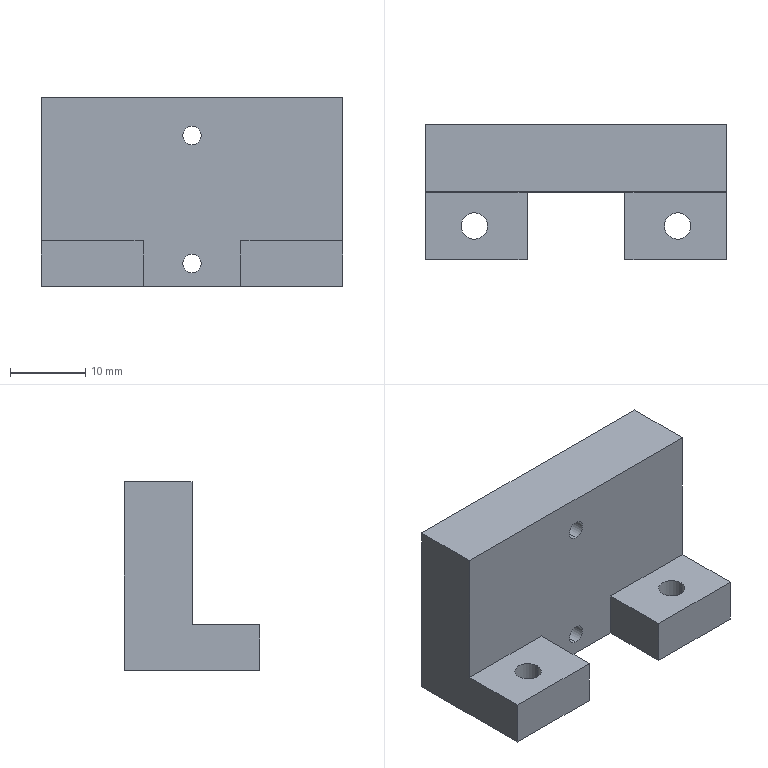Part | SolidWorks | features BaseBody 1 | 1 solid | 20 faces | box 40 x 18 x 25 mm | volume 10257 mm3 | plane 12 | cylinder 8 | commonest cylinder face diameters 2.459 x4 3.5 x4
STEP:
#1=CARTESIAN_POINT('',(-20.,18.,21.23));
#2=VERTEX_POINT('',#1);
#3=CARTESIAN_POINT('',(-20.,18.,18.77));
#4=VERTEX_POINT('',#3);
#5=CARTESIAN_POINT('',(-20.,18.,20.));
#6=DIRECTION('',(0.,-1.,0.));
#7=DIRECTION('',(0.,0.,-1.));
#8=AXIS2_PLACEMENT_3D('',#5,#6,#7);
#9=CIRCLE('',#8,1.23);
#10=EDGE_CURVE('',#2,#4,#9,.T.);
#11=ORIENTED_EDGE('',*,*,#10,.F.);
#12=CARTESIAN_POINT('',(-20.,9.,21.23));
#13=VERTEX_POINT('',#12);
#14=CARTESIAN_POINT('',(-20.,59.488,21.23));
#15=DIRECTION('',(0.,-1.,0.));
#16=VECTOR('',#15,1000.);
#17=LINE('',#14,#16);
#18=EDGE_CURVE('',#2,#13,#17,.T.);
#19=ORIENTED_EDGE('',*,*,#18,.T.);
#20=CARTESIAN_POINT('',(-20.,9.,18.77));
#21=VERTEX_POINT('',#20);
#22=CARTESIAN_POINT('',(-20.,9.,20.));
#23=DIRECTION('',(0.,1.,0.));
#24=DIRECTION('',(0.,0.,-1.));
#25=AXIS2_PLACEMENT_3D('',#22,#23,#24);
#26=CIRCLE('',#25,1.23);
#27=EDGE_CURVE('',#21,#13,#26,.T.);
#28=ORIENTED_EDGE('',*,*,#27,.F.);
#29=CARTESIAN_POINT('',(-20.,59.488,18.771));
#30=DIRECTION('',(0.,-1.,0.));
#31=VECTOR('',#30,1000.);
#32=LINE('',#29,#31);
#33=EDGE_CURVE('',#4,#21,#32,.T.);
#34=ORIENTED_EDGE('',*,*,#33,.F.);
#35=EDGE_LOOP('',(#11,#19,#28,#34));
#36=FACE_OUTER_BOUND('',#35,.T.);
#37=CARTESIAN_POINT('',(-20.,59.488,20.));
#38=DIRECTION('',(0.,-1.,0.));
#39=DIRECTION('',(0.,0.,-1.));
#40=AXIS2_PLACEMENT_3D('',#37,#38,#39);
#41=CYLINDRICAL_SURFACE('',#40,1.23);
#42=ADVANCED_FACE('',(#36),#41,.F.);
#43=CARTESIAN_POINT('',(-20.,18.,4.23));
#44=VERTEX_POINT('',#43);
#45=CARTESIAN_POINT('',(-20.,18.,1.771));
#46=VERTEX_POINT('',#45);
#47=CARTESIAN_POINT('',(-20.,18.,3.));
#48=DIRECTION('',(0.,-1.,0.));
#49=DIRECTION('',(0.,0.,-1.));
#50=AXIS2_PLACEMENT_3D('',#47,#48,#49);
#51=CIRCLE('',#50,1.23);
#52=EDGE_CURVE('',#44,#46,#51,.T.);
#53=ORIENTED_EDGE('',*,*,#52,.F.);
#54=CARTESIAN_POINT('',(-20.,9.,4.23));
#55=VERTEX_POINT('',#54);
#56=CARTESIAN_POINT('',(-20.,59.488,4.23));
#57=DIRECTION('',(0.,-1.,0.));
#58=VECTOR('',#57,1000.);
#59=LINE('',#56,#58);
#60=EDGE_CURVE('',#44,#55,#59,.T.);
#61=ORIENTED_EDGE('',*,*,#60,.T.);
#62=CARTESIAN_POINT('',(-20.,9.,1.77));
#63=VERTEX_POINT('',#62);
#64=CARTESIAN_POINT('',(-20.,9.,3.));
#65=DIRECTION('',(0.,1.,0.));
#66=DIRECTION('',(0.,0.,-1.));
#67=AXIS2_PLACEMENT_3D('',#64,#65,#66);
#68=CIRCLE('',#67,1.23);
#69=EDGE_CURVE('',#63,#55,#68,.T.);
#70=ORIENTED_EDGE('',*,*,#69,.F.);
#71=CARTESIAN_POINT('',(-20.,59.488,1.771));
#72=DIRECTION('',(0.,-1.,0.));
#73=VECTOR('',#72,1000.);
#74=LINE('',#71,#73);
#75=EDGE_CURVE('',#46,#63,#74,.T.);
#76=ORIENTED_EDGE('',*,*,#75,.F.);
#77=EDGE_LOOP('',(#53,#61,#70,#76));
#78=FACE_OUTER_BOUND('',#77,.T.);
#79=CARTESIAN_POINT('',(-20.,59.488,3.));
#80=DIRECTION('',(0.,-1.,0.));
#81=DIRECTION('',(0.,0.,-1.));
#82=AXIS2_PLACEMENT_3D('',#79,#80,#81);
#83=CYLINDRICAL_SURFACE('',#82,1.23);
#84=ADVANCED_FACE('',(#78),#83,.F.);
#85=CARTESIAN_POINT('',(-4.75,4.5,0.));
#86=VERTEX_POINT('',#85);
#87=CARTESIAN_POINT('',(-8.25,4.5,0.));
#88=VERTEX_POINT('',#87);
#89=CARTESIAN_POINT('',(-6.5,4.5,0.));
#90=DIRECTION('',(0.,0.,-1.));
#91=DIRECTION('',(1.,0.,0.));
#92=AXIS2_PLACEMENT_3D('',#89,#90,#91);
#93=CIRCLE('',#92,1.75);
#94=EDGE_CURVE('',#86,#88,#93,.T.);
#95=ORIENTED_EDGE('',*,*,#94,.T.);
#96=CARTESIAN_POINT('',(-8.25,4.5,6.));
#97=VERTEX_POINT('',#96);
#98=CARTESIAN_POINT('',(-8.25,4.5,-44.488));
#99=DIRECTION('',(0.,0.,1.));
#100=VECTOR('',#99,1000.);
#101=LINE('',#98,#100);
#102=EDGE_CURVE('',#88,#97,#101,.T.);
#103=ORIENTED_EDGE('',*,*,#102,.T.);
#104=CARTESIAN_POINT('',(-4.75,4.5,6.));
#105=VERTEX_POINT('',#104);
#106=CARTESIAN_POINT('',(-6.5,4.5,6.));
#107=DIRECTION('',(0.,0.,-1.));
#108=DIRECTION('',(1.,0.,0.));
#109=AXIS2_PLACEMENT_3D('',#106,#107,#108);
#110=CIRCLE('',#109,1.75);
#111=EDGE_CURVE('',#105,#97,#110,.T.);
#112=ORIENTED_EDGE('',*,*,#111,.F.);
#113=CARTESIAN_POINT('',(-4.75,4.5,-44.488));
#114=DIRECTION('',(0.,0.,1.));
#115=VECTOR('',#114,1000.);
#116=LINE('',#113,#115);
#117=EDGE_CURVE('',#86,#105,#116,.T.);
#118=ORIENTED_EDGE('',*,*,#117,.F.);
#119=EDGE_LOOP('',(#95,#103,#112,#118));
#120=FACE_OUTER_BOUND('',#119,.T.);
#121=CARTESIAN_POINT('',(-6.5,4.5,-44.488));
#122=DIRECTION('',(0.,0.,1.));
#123=DIRECTION('',(1.,0.,0.));
#124=AXIS2_PLACEMENT_3D('',#121,#122,#123);
#125=CYLINDRICAL_SURFACE('',#124,1.75);
#126=ADVANCED_FACE('',(#120),#125,.F.);
#127=CARTESIAN_POINT('',(-31.75,4.5,0.));
#128=VERTEX_POINT('',#127);
#129=CARTESIAN_POINT('',(-35.25,4.5,0.));
#130=VERTEX_POINT('',#129);
#131=CARTESIAN_POINT('',(-33.5,4.5,0.));
#132=DIRECTION('',(0.,0.,-1.));
#133=DIRECTION('',(1.,0.,0.));
#134=AXIS2_PLACEMENT_3D('',#131,#132,#133);
#135=CIRCLE('',#134,1.75);
#136=EDGE_CURVE('',#128,#130,#135,.T.);
#137=ORIENTED_EDGE('',*,*,#136,.T.);
#138=CARTESIAN_POINT('',(-35.25,4.5,6.));
#139=VERTEX_POINT('',#138);
#140=CARTESIAN_POINT('',(-35.25,4.5,-44.488));
#141=DIRECTION('',(0.,0.,1.));
#142=VECTOR('',#141,1000.);
#143=LINE('',#140,#142);
#144=EDGE_CURVE('',#130,#139,#143,.T.);
#145=ORIENTED_EDGE('',*,*,#144,.T.);
#146=CARTESIAN_POINT('',(-31.75,4.5,6.));
#147=VERTEX_POINT('',#146);
#148=CARTESIAN_POINT('',(-33.5,4.5,6.));
#149=DIRECTION('',(0.,0.,1.));
#150=DIRECTION('',(1.,0.,0.));
#151=AXIS2_PLACEMENT_3D('',#148,#149,#150);
#152=CIRCLE('',#151,1.75);
#153=EDGE_CURVE('',#139,#147,#152,.T.);
#154=ORIENTED_EDGE('',*,*,#153,.T.);
#155=CARTESIAN_POINT('',(-31.75,4.5,-44.488));
#156=DIRECTION('',(0.,0.,1.));
#157=VECTOR('',#156,1000.);
#158=LINE('',#155,#157);
#159=EDGE_CURVE('',#128,#147,#158,.T.);
#160=ORIENTED_EDGE('',*,*,#159,.F.);
#161=EDGE_LOOP('',(#137,#145,#154,#160));
#162=FACE_OUTER_BOUND('',#161,.T.);
#163=CARTESIAN_POINT('',(-33.5,4.5,-44.488));
#164=DIRECTION('',(0.,0.,1.));
#165=DIRECTION('',(1.,0.,0.));
#166=AXIS2_PLACEMENT_3D('',#163,#164,#165);
#167=CYLINDRICAL_SURFACE('',#166,1.75);
#168=ADVANCED_FACE('',(#162),#167,.F.);
#169=CARTESIAN_POINT('',(-20.,18.,20.));
#170=DIRECTION('',(0.,-1.,0.));
#171=DIRECTION('',(0.,0.,-1.));
#172=AXIS2_PLACEMENT_3D('',#169,#170,#171);
#173=CIRCLE('',#172,1.23);
#174=EDGE_CURVE('',#4,#2,#173,.T.);
#175=ORIENTED_EDGE('',*,*,#174,.T.);
#176=ORIENTED_EDGE('',*,*,#10,.T.);
#177=EDGE_LOOP('',(#175,#176));
#178=FACE_BOUND('',#177,.T.);
#179=CARTESIAN_POINT('',(-20.,18.,3.));
#180=DIRECTION('',(0.,-1.,0.));
#181=DIRECTION('',(0.,0.,-1.));
#182=AXIS2_PLACEMENT_3D('',#179,#180,#181);
#183=CIRCLE('',#182,1.23);
#184=EDGE_CURVE('',#46,#44,#183,.T.);
#185=ORIENTED_EDGE('',*,*,#184,.T.);
#186=ORIENTED_EDGE('',*,*,#52,.T.);
#187=EDGE_LOOP('',(#185,#186));
#188=FACE_BOUND('',#187,.T.);
#189=CARTESIAN_POINT('',(-40.,18.,0.));
#190=VERTEX_POINT('',#189);
#191=CARTESIAN_POINT('',(-40.,18.,25.));
#192=VERTEX_POINT('',#191);
#193=CARTESIAN_POINT('',(-40.,18.,0.));
#194=DIRECTION('',(0.,0.,1.));
#195=VECTOR('',#194,1000.);
#196=LINE('',#193,#195);
#197=EDGE_CURVE('',#190,#192,#196,.T.);
#198=ORIENTED_EDGE('',*,*,#197,.T.);
#199=CARTESIAN_POINT('',(0.,18.,25.));
#200=VERTEX_POINT('',#199);
#201=CARTESIAN_POINT('',(-40.,18.,25.));
#202=DIRECTION('',(1.,0.,0.));
#203=VECTOR('',#202,1000.);
#204=LINE('',#201,#203);
#205=EDGE_CURVE('',#192,#200,#204,.T.);
#206=ORIENTED_EDGE('',*,*,#205,.T.);
#207=CARTESIAN_POINT('',(0.,18.,0.));
#208=VERTEX_POINT('',#207);
#209=CARTESIAN_POINT('',(0.,18.,0.));
#210=DIRECTION('',(0.,0.,-1.));
#211=VECTOR('',#210,1000.);
#212=LINE('',#209,#211);
#213=EDGE_CURVE('',#200,#208,#212,.T.);
#214=ORIENTED_EDGE('',*,*,#213,.T.);
#215=CARTESIAN_POINT('',(-40.,18.,0.));
#216=DIRECTION('',(-1.,0.,0.));
#217=VECTOR('',#216,1000.);
#218=LINE('',#215,#217);
#219=EDGE_CURVE('',#208,#190,#218,.T.);
#220=ORIENTED_EDGE('',*,*,#219,.T.);
#221=EDGE_LOOP('',(#198,#206,#214,#220));
#222=FACE_OUTER_BOUND('',#221,.T.);
#223=CARTESIAN_POINT('',(-40.,18.,0.));
#224=DIRECTION('',(0.,1.,0.));
#225=DIRECTION('',(0.,0.,1.));
#226=AXIS2_PLACEMENT_3D('',#223,#224,#225);
#227=PLANE('',#226);
#228=ADVANCED_FACE('',(#178,#188,#222),#227,.T.);
#229=ORIENTED_EDGE('',*,*,#18,.F.);
#230=ORIENTED_EDGE('',*,*,#174,.F.);
#231=ORIENTED_EDGE('',*,*,#33,.T.);
#232=CARTESIAN_POINT('',(-20.,9.,20.));
#233=DIRECTION('',(0.,1.,0.));
#234=DIRECTION('',(0.,0.,-1.));
#235=AXIS2_PLACEMENT_3D('',#232,#233,#234);
#236=CIRCLE('',#235,1.23);
#237=EDGE_CURVE('',#13,#21,#236,.T.);
#238=ORIENTED_EDGE('',*,*,#237,.F.);
#239=EDGE_LOOP('',(#229,#230,#231,#238));
#240=FACE_OUTER_BOUND('',#239,.T.);
#241=CARTESIAN_POINT('',(-20.,59.488,20.));
#242=DIRECTION('',(0.,-1.,0.));
#243=DIRECTION('',(0.,0.,-1.));
#244=AXIS2_PLACEMENT_3D('',#241,#242,#243);
#245=CYLINDRICAL_SURFACE('',#244,1.23);
#246=ADVANCED_FACE('',(#240),#245,.F.);
#247=ORIENTED_EDGE('',*,*,#60,.F.);
#248=ORIENTED_EDGE('',*,*,#184,.F.);
#249=ORIENTED_EDGE('',*,*,#75,.T.);
#250=CARTESIAN_POINT('',(-20.,9.,3.));
#251=DIRECTION('',(0.,1.,0.));
#252=DIRECTION('',(0.,0.,-1.));
#253=AXIS2_PLACEMENT_3D('',#250,#251,#252);
#254=CIRCLE('',#253,1.23);
#255=EDGE_CURVE('',#55,#63,#254,.T.);
#256=ORIENTED_EDGE('',*,*,#255,.F.);
#257=EDGE_LOOP('',(#247,#248,#249,#256));
#258=FACE_OUTER_BOUND('',#257,.T.);
#259=CARTESIAN_POINT('',(-20.,59.488,3.));
#260=DIRECTION('',(0.,-1.,0.));
#261=DIRECTION('',(0.,0.,-1.));
#262=AXIS2_PLACEMENT_3D('',#259,#260,#261);
#263=CYLINDRICAL_SURFACE('',#262,1.23);
#264=ADVANCED_FACE('',(#258),#263,.F.);
#265=CARTESIAN_POINT('',(0.,9.,25.));
#266=VERTEX_POINT('',#265);
#267=CARTESIAN_POINT('',(0.,13.5,25.));
#268=DIRECTION('',(0.,1.,0.));
#269=VECTOR('',#268,1000.);
#270=LINE('',#267,#269);
#271=EDGE_CURVE('',#266,#200,#270,.T.);
#272=ORIENTED_EDGE('',*,*,#271,.T.);
#273=ORIENTED_EDGE('',*,*,#205,.F.);
#274=CARTESIAN_POINT('',(-40.,9.,25.));
#275=VERTEX_POINT('',#274);
#276=CARTESIAN_POINT('',(-40.,13.5,25.));
#277=DIRECTION('',(0.,-1.,0.));
#278=VECTOR('',#277,1000.);
#279=LINE('',#276,#278);
#280=EDGE_CURVE('',#192,#275,#279,.T.);
#281=ORIENTED_EDGE('',*,*,#280,.T.);
#282=CARTESIAN_POINT('',(-20.,9.,25.));
#283=DIRECTION('',(1.,0.,0.));
#284=VECTOR('',#283,1000.);
#285=LINE('',#282,#284);
#286=EDGE_CURVE('',#275,#266,#285,.T.);
#287=ORIENTED_EDGE('',*,*,#286,.T.);
#288=EDGE_LOOP('',(#272,#273,#281,#287));
#289=FACE_OUTER_BOUND('',#288,.T.);
#290=CARTESIAN_POINT('',(-20.,13.5,25.));
#291=DIRECTION('',(0.,0.,1.));
#292=DIRECTION('',(1.,0.,0.));
#293=AXIS2_PLACEMENT_3D('',#290,#291,#292);
#294=PLANE('',#293);
#295=ADVANCED_FACE('',(#289),#294,.T.);
#296=CARTESIAN_POINT('',(-40.,0.,0.));
#297=VERTEX_POINT('',#296);
#298=CARTESIAN_POINT('',(-40.,0.,6.));
#299=VERTEX_POINT('',#298);
#300=CARTESIAN_POINT('',(-40.,0.,0.));
#301=DIRECTION('',(0.,0.,1.));
#302=VECTOR('',#301,1000.);
#303=LINE('',#300,#302);
#304=EDGE_CURVE('',#297,#299,#303,.T.);
#305=ORIENTED_EDGE('',*,*,#304,.T.);
#306=CARTESIAN_POINT('',(-40.,9.,6.));
#307=VERTEX_POINT('',#306);
#308=CARTESIAN_POINT('',(-40.,0.,6.));
#309=DIRECTION('',(0.,1.,0.));
#310=VECTOR('',#309,1000.);
#311=LINE('',#308,#310);
#312=EDGE_CURVE('',#299,#307,#311,.T.);
#313=ORIENTED_EDGE('',*,*,#312,.T.);
#314=CARTESIAN_POINT('',(-40.,9.,0.));
#315=DIRECTION('',(0.,0.,1.));
#316=VECTOR('',#315,1000.);
#317=LINE('',#314,#316);
#318=EDGE_CURVE('',#307,#275,#317,.T.);
#319=ORIENTED_EDGE('',*,*,#318,.T.);
#320=ORIENTED_EDGE('',*,*,#280,.F.);
#321=ORIENTED_EDGE('',*,*,#197,.F.);
#322=CARTESIAN_POINT('',(-40.,0.,0.));
#323=DIRECTION('',(0.,-1.,0.));
#324=VECTOR('',#323,1000.);
#325=LINE('',#322,#324);
#326=EDGE_CURVE('',#190,#297,#325,.T.);
#327=ORIENTED_EDGE('',*,*,#326,.T.);
#328=EDGE_LOOP('',(#305,#313,#319,#320,#321,#327));
#329=FACE_OUTER_BOUND('',#328,.T.);
#330=CARTESIAN_POINT('',(-40.,0.,0.));
#331=DIRECTION('',(-1.,0.,0.));
#332=DIRECTION('',(0.,0.,1.));
#333=AXIS2_PLACEMENT_3D('',#330,#331,#332);
#334=PLANE('',#333);
#335=ADVANCED_FACE('',(#329),#334,.T.);
#336=ORIENTED_EDGE('',*,*,#94,.F.);
#337=CARTESIAN_POINT('',(-6.5,4.5,0.));
#338=DIRECTION('',(0.,0.,-1.));
#339=DIRECTION('',(1.,0.,0.));
#340=AXIS2_PLACEMENT_3D('',#337,#338,#339);
#341=CIRCLE('',#340,1.75);
#342=EDGE_CURVE('',#88,#86,#341,.T.);
#343=ORIENTED_EDGE('',*,*,#342,.F.);
#344=EDGE_LOOP('',(#336,#343));
#345=FACE_BOUND('',#344,.T.);
#346=ORIENTED_EDGE('',*,*,#136,.F.);
#347=CARTESIAN_POINT('',(-33.5,4.5,0.));
#348=DIRECTION('',(0.,0.,-1.));
#349=DIRECTION('',(1.,0.,0.));
#350=AXIS2_PLACEMENT_3D('',#347,#348,#349);
#351=CIRCLE('',#350,1.75);
#352=EDGE_CURVE('',#130,#128,#351,.T.);
#353=ORIENTED_EDGE('',*,*,#352,.F.);
#354=EDGE_LOOP('',(#346,#353));
#355=FACE_BOUND('',#354,.T.);
#356=CARTESIAN_POINT('',(-26.5,0.,0.));
#357=VERTEX_POINT('',#356);
#358=CARTESIAN_POINT('',(-20.,0.,0.));
#359=DIRECTION('',(1.,0.,0.));
#360=VECTOR('',#359,1000.);
#361=LINE('',#358,#360);
#362=EDGE_CURVE('',#297,#357,#361,.T.);
#363=ORIENTED_EDGE('',*,*,#362,.F.);
#364=ORIENTED_EDGE('',*,*,#326,.F.);
#365=ORIENTED_EDGE('',*,*,#219,.F.);
#366=CARTESIAN_POINT('',(0.,0.,0.));
#367=VERTEX_POINT('',#366);
#368=CARTESIAN_POINT('',(0.,9.,0.));
#369=DIRECTION('',(0.,1.,0.));
#370=VECTOR('',#369,1000.);
#371=LINE('',#368,#370);
#372=EDGE_CURVE('',#367,#208,#371,.T.);
#373=ORIENTED_EDGE('',*,*,#372,.F.);
#374=CARTESIAN_POINT('',(-13.5,0.,0.));
#375=VERTEX_POINT('',#374);
#376=CARTESIAN_POINT('',(-20.,0.,0.));
#377=DIRECTION('',(1.,0.,0.));
#378=VECTOR('',#377,1000.);
#379=LINE('',#376,#378);
#380=EDGE_CURVE('',#375,#367,#379,.T.);
#381=ORIENTED_EDGE('',*,*,#380,.F.);
#382=CARTESIAN_POINT('',(-13.5,9.,0.));
#383=VERTEX_POINT('',#382);
#384=CARTESIAN_POINT('',(-13.5,9.,0.));
#385=DIRECTION('',(0.,-1.,0.));
#386=VECTOR('',#385,1000.);
#387=LINE('',#384,#386);
#388=EDGE_CURVE('',#383,#375,#387,.T.);
#389=ORIENTED_EDGE('',*,*,#388,.F.);
#390=CARTESIAN_POINT('',(-26.5,9.,0.));
#391=VERTEX_POINT('',#390);
#392=CARTESIAN_POINT('',(-20.,9.,0.));
#393=DIRECTION('',(1.,0.,0.));
#394=VECTOR('',#393,1000.);
#395=LINE('',#392,#394);
#396=EDGE_CURVE('',#391,#383,#395,.T.);
#397=ORIENTED_EDGE('',*,*,#396,.F.);
#398=CARTESIAN_POINT('',(-26.5,9.,0.));
#399=DIRECTION('',(0.,1.,0.));
#400=VECTOR('',#399,1000.);
#401=LINE('',#398,#400);
#402=EDGE_CURVE('',#357,#391,#401,.T.);
#403=ORIENTED_EDGE('',*,*,#402,.F.);
#404=EDGE_LOOP('',(#363,#364,#365,#373,#381,#389,#397,#403));
#405=FACE_OUTER_BOUND('',#404,.T.);
#406=CARTESIAN_POINT('',(-20.,9.,0.));
#407=DIRECTION('',(0.,0.,1.));
#408=DIRECTION('',(1.,0.,0.));
#409=AXIS2_PLACEMENT_3D('',#406,#407,#408);
#410=PLANE('',#409);
#411=ADVANCED_FACE('',(#345,#355,#405),#410,.F.);
#412=ORIENTED_EDGE('',*,*,#271,.F.);
#413=CARTESIAN_POINT('',(0.,9.,6.));
#414=VERTEX_POINT('',#413);
#415=CARTESIAN_POINT('',(0.,9.,0.));
#416=DIRECTION('',(0.,0.,-1.));
#417=VECTOR('',#416,1000.);
#418=LINE('',#415,#417);
#419=EDGE_CURVE('',#266,#414,#418,.T.);
#420=ORIENTED_EDGE('',*,*,#419,.T.);
#421=CARTESIAN_POINT('',(0.,0.,6.));
#422=VERTEX_POINT('',#421);
#423=CARTESIAN_POINT('',(0.,18.,6.));
#424=DIRECTION('',(0.,-1.,0.));
#425=VECTOR('',#424,1000.);
#426=LINE('',#423,#425);
#427=EDGE_CURVE('',#414,#422,#426,.T.);
#428=ORIENTED_EDGE('',*,*,#427,.T.);
#429=CARTESIAN_POINT('',(0.,0.,0.));
#430=DIRECTION('',(0.,0.,-1.));
#431=VECTOR('',#430,1000.);
#432=LINE('',#429,#431);
#433=EDGE_CURVE('',#422,#367,#432,.T.);
#434=ORIENTED_EDGE('',*,*,#433,.T.);
#435=ORIENTED_EDGE('',*,*,#372,.T.);
#436=ORIENTED_EDGE('',*,*,#213,.F.);
#437=EDGE_LOOP('',(#412,#420,#428,#434,#435,#436));
#438=FACE_OUTER_BOUND('',#437,.T.);
#439=CARTESIAN_POINT('',(0.,18.,0.));
#440=DIRECTION('',(1.,0.,0.));
#441=DIRECTION('',(0.,0.,-1.));
#442=AXIS2_PLACEMENT_3D('',#439,#440,#441);
#443=PLANE('',#442);
#444=ADVANCED_FACE('',(#438),#443,.T.);
#445=ORIENTED_EDGE('',*,*,#27,.T.);
#446=ORIENTED_EDGE('',*,*,#237,.T.);
#447=EDGE_LOOP('',(#445,#446));
#448=FACE_BOUND('',#447,.T.);
#449=ORIENTED_EDGE('',*,*,#69,.T.);
#450=ORIENTED_EDGE('',*,*,#255,.T.);
#451=EDGE_LOOP('',(#449,#450));
#452=FACE_BOUND('',#451,.T.);
#453=CARTESIAN_POINT('',(-26.5,9.,6.));
#454=VERTEX_POINT('',#453);
#455=CARTESIAN_POINT('',(0.,9.,6.));
#456=DIRECTION('',(-1.,0.,0.));
#457=VECTOR('',#456,1000.);
#458=LINE('',#455,#457);
#459=EDGE_CURVE('',#454,#307,#458,.T.);
#460=ORIENTED_EDGE('',*,*,#459,.F.);
#461=CARTESIAN_POINT('',(-26.5,9.,6.));
#462=DIRECTION('',(0.,0.,1.));
#463=VECTOR('',#462,1000.);
#464=LINE('',#461,#463);
#465=EDGE_CURVE('',#391,#454,#464,.T.);
#466=ORIENTED_EDGE('',*,*,#465,.F.);
#467=ORIENTED_EDGE('',*,*,#396,.T.);
#468=CARTESIAN_POINT('',(-13.5,9.,6.));
#469=VERTEX_POINT('',#468);
#470=CARTESIAN_POINT('',(-13.5,9.,6.));
#471=DIRECTION('',(0.,0.,-1.));
#472=VECTOR('',#471,1000.);
#473=LINE('',#470,#472);
#474=EDGE_CURVE('',#469,#383,#473,.T.);
#475=ORIENTED_EDGE('',*,*,#474,.F.);
#476=CARTESIAN_POINT('',(0.,9.,6.));
#477=DIRECTION('',(-1.,0.,0.));
#478=VECTOR('',#477,1000.);
#479=LINE('',#476,#478);
#480=EDGE_CURVE('',#414,#469,#479,.T.);
#481=ORIENTED_EDGE('',*,*,#480,.F.);
#482=ORIENTED_EDGE('',*,*,#419,.F.);
#483=ORIENTED_EDGE('',*,*,#286,.F.);
#484=ORIENTED_EDGE('',*,*,#318,.F.);
#485=EDGE_LOOP('',(#460,#466,#467,#475,#481,#482,#483,#484));
#486=FACE_OUTER_BOUND('',#485,.T.);
#487=CARTESIAN_POINT('',(0.,9.,6.));
#488=DIRECTION('',(0.,1.,0.));
#489=DIRECTION('',(0.,0.,1.));
#490=AXIS2_PLACEMENT_3D('',#487,#488,#489);
#491=PLANE('',#490);
#492=ADVANCED_FACE('',(#448,#452,#486),#491,.F.);
#493=CARTESIAN_POINT('',(-33.5,4.5,6.));
#494=DIRECTION('',(0.,0.,1.));
#495=DIRECTION('',(1.,0.,0.));
#496=AXIS2_PLACEMENT_3D('',#493,#494,#495);
#497=CIRCLE('',#496,1.75);
#498=EDGE_CURVE('',#147,#139,#497,.T.);
#499=ORIENTED_EDGE('',*,*,#498,.F.);
#500=ORIENTED_EDGE('',*,*,#153,.F.);
#501=EDGE_LOOP('',(#499,#500));
#502=FACE_BOUND('',#501,.T.);
#503=ORIENTED_EDGE('',*,*,#459,.T.);
#504=ORIENTED_EDGE('',*,*,#312,.F.);
#505=CARTESIAN_POINT('',(-26.5,0.,6.));
#506=VERTEX_POINT('',#505);
#507=CARTESIAN_POINT('',(0.,0.,6.));
#508=DIRECTION('',(-1.,0.,0.));
#509=VECTOR('',#508,1000.);
#510=LINE('',#507,#509);
#511=EDGE_CURVE('',#506,#299,#510,.T.);
#512=ORIENTED_EDGE('',*,*,#511,.F.);
#513=CARTESIAN_POINT('',(-26.5,0.,6.));
#514=DIRECTION('',(0.,-1.,0.));
#515=VECTOR('',#514,1000.);
#516=LINE('',#513,#515);
#517=EDGE_CURVE('',#454,#506,#516,.T.);
#518=ORIENTED_EDGE('',*,*,#517,.F.);
#519=EDGE_LOOP('',(#503,#504,#512,#518));
#520=FACE_OUTER_BOUND('',#519,.T.);
#521=CARTESIAN_POINT('',(0.,0.,6.));
#522=DIRECTION('',(0.,0.,-1.));
#523=DIRECTION('',(-1.,0.,0.));
#524=AXIS2_PLACEMENT_3D('',#521,#522,#523);
#525=PLANE('',#524);
#526=ADVANCED_FACE('',(#502,#520),#525,.F.);
#527=ORIENTED_EDGE('',*,*,#304,.F.);
#528=ORIENTED_EDGE('',*,*,#362,.T.);
#529=CARTESIAN_POINT('',(-26.5,0.,0.));
#530=DIRECTION('',(0.,0.,1.));
#531=VECTOR('',#530,1000.);
#532=LINE('',#529,#531);
#533=EDGE_CURVE('',#357,#506,#532,.T.);
#534=ORIENTED_EDGE('',*,*,#533,.T.);
#535=ORIENTED_EDGE('',*,*,#511,.T.);
#536=EDGE_LOOP('',(#527,#528,#534,#535));
#537=FACE_OUTER_BOUND('',#536,.T.);
#538=CARTESIAN_POINT('',(0.,0.,0.));
#539=DIRECTION('',(0.,-1.,0.));
#540=DIRECTION('',(0.,0.,-1.));
#541=AXIS2_PLACEMENT_3D('',#538,#539,#540);
#542=PLANE('',#541);
#543=ADVANCED_FACE('',(#537),#542,.T.);
#544=ORIENTED_EDGE('',*,*,#102,.F.);
#545=ORIENTED_EDGE('',*,*,#342,.T.);
#546=ORIENTED_EDGE('',*,*,#117,.T.);
#547=CARTESIAN_POINT('',(-6.5,4.5,6.));
#548=DIRECTION('',(0.,0.,-1.));
#549=DIRECTION('',(1.,0.,0.));
#550=AXIS2_PLACEMENT_3D('',#547,#548,#549);
#551=CIRCLE('',#550,1.75);
#552=EDGE_CURVE('',#97,#105,#551,.T.);
#553=ORIENTED_EDGE('',*,*,#552,.F.);
#554=EDGE_LOOP('',(#544,#545,#546,#553));
#555=FACE_OUTER_BOUND('',#554,.T.);
#556=CARTESIAN_POINT('',(-6.5,4.5,-44.488));
#557=DIRECTION('',(0.,0.,1.));
#558=DIRECTION('',(1.,0.,0.));
#559=AXIS2_PLACEMENT_3D('',#556,#557,#558);
#560=CYLINDRICAL_SURFACE('',#559,1.75);
#561=ADVANCED_FACE('',(#555),#560,.F.);
#562=ORIENTED_EDGE('',*,*,#144,.F.);
#563=ORIENTED_EDGE('',*,*,#352,.T.);
#564=ORIENTED_EDGE('',*,*,#159,.T.);
#565=ORIENTED_EDGE('',*,*,#498,.T.);
#566=EDGE_LOOP('',(#562,#563,#564,#565));
#567=FACE_OUTER_BOUND('',#566,.T.);
#568=CARTESIAN_POINT('',(-33.5,4.5,-44.488));
#569=DIRECTION('',(0.,0.,1.));
#570=DIRECTION('',(1.,0.,0.));
#571=AXIS2_PLACEMENT_3D('',#568,#569,#570);
#572=CYLINDRICAL_SURFACE('',#571,1.75);
#573=ADVANCED_FACE('',(#567),#572,.F.);
#574=ORIENTED_EDGE('',*,*,#517,.T.);
#575=ORIENTED_EDGE('',*,*,#533,.F.);
#576=ORIENTED_EDGE('',*,*,#402,.T.);
#577=ORIENTED_EDGE('',*,*,#465,.T.);
#578=EDGE_LOOP('',(#574,#575,#576,#577));
#579=FACE_OUTER_BOUND('',#578,.T.);
#580=CARTESIAN_POINT('',(-26.5,0.,6.));
#581=DIRECTION('',(-1.,0.,0.));
#582=DIRECTION('',(0.,0.,1.));
#583=AXIS2_PLACEMENT_3D('',#580,#581,#582);
#584=PLANE('',#583);
#585=ADVANCED_FACE('',(#579),#584,.F.);
#586=ORIENTED_EDGE('',*,*,#433,.F.);
#587=CARTESIAN_POINT('',(-13.5,0.,6.));
#588=VERTEX_POINT('',#587);
#589=CARTESIAN_POINT('',(0.,0.,6.));
#590=DIRECTION('',(-1.,0.,0.));
#591=VECTOR('',#590,1000.);
#592=LINE('',#589,#591);
#593=EDGE_CURVE('',#422,#588,#592,.T.);
#594=ORIENTED_EDGE('',*,*,#593,.T.);
#595=CARTESIAN_POINT('',(-13.5,0.,0.));
#596=DIRECTION('',(0.,0.,-1.));
#597=VECTOR('',#596,1000.);
#598=LINE('',#595,#597);
#599=EDGE_CURVE('',#588,#375,#598,.T.);
#600=ORIENTED_EDGE('',*,*,#599,.T.);
#601=ORIENTED_EDGE('',*,*,#380,.T.);
#602=EDGE_LOOP('',(#586,#594,#600,#601));
#603=FACE_OUTER_BOUND('',#602,.T.);
#604=CARTESIAN_POINT('',(0.,0.,0.));
#605=DIRECTION('',(0.,-1.,0.));
#606=DIRECTION('',(0.,0.,-1.));
#607=AXIS2_PLACEMENT_3D('',#604,#605,#606);
#608=PLANE('',#607);
#609=ADVANCED_FACE('',(#603),#608,.T.);
#610=ORIENTED_EDGE('',*,*,#388,.T.);
#611=ORIENTED_EDGE('',*,*,#599,.F.);
#612=CARTESIAN_POINT('',(-13.5,0.,6.));
#613=DIRECTION('',(0.,-1.,0.));
#614=VECTOR('',#613,1000.);
#615=LINE('',#612,#614);
#616=EDGE_CURVE('',#469,#588,#615,.T.);
#617=ORIENTED_EDGE('',*,*,#616,.F.);
#618=ORIENTED_EDGE('',*,*,#474,.T.);
#619=EDGE_LOOP('',(#610,#611,#617,#618));
#620=FACE_OUTER_BOUND('',#619,.T.);
#621=CARTESIAN_POINT('',(-13.5,0.,0.));
#622=DIRECTION('',(1.,0.,0.));
#623=DIRECTION('',(0.,0.,-1.));
#624=AXIS2_PLACEMENT_3D('',#621,#622,#623);
#625=PLANE('',#624);
#626=ADVANCED_FACE('',(#620),#625,.F.);
#627=ORIENTED_EDGE('',*,*,#111,.T.);
#628=ORIENTED_EDGE('',*,*,#552,.T.);
#629=EDGE_LOOP('',(#627,#628));
#630=FACE_BOUND('',#629,.T.);
#631=ORIENTED_EDGE('',*,*,#593,.F.);
#632=ORIENTED_EDGE('',*,*,#427,.F.);
#633=ORIENTED_EDGE('',*,*,#480,.T.);
#634=ORIENTED_EDGE('',*,*,#616,.T.);
#635=EDGE_LOOP('',(#631,#632,#633,#634));
#636=FACE_OUTER_BOUND('',#635,.T.);
#637=CARTESIAN_POINT('',(0.,0.,6.));
#638=DIRECTION('',(0.,0.,-1.));
#639=DIRECTION('',(-1.,0.,0.));
#640=AXIS2_PLACEMENT_3D('',#637,#638,#639);
#641=PLANE('',#640);
#642=ADVANCED_FACE('',(#630,#636),#641,.F.);
#643=CLOSED_SHELL('',(#42,#84,#126,#168,#228,#246,#264,#295,#335,#411,#444,#492,#526,#543,#561,#573,#585,#609,#626,#642));
#644=MANIFOLD_SOLID_BREP('',#643);
#645=CARTESIAN_POINT('',(0.,0.,0.));
#646=DIRECTION('',(0.,0.,1.));
#647=DIRECTION('',(1.,0.,0.));
#648=AXIS2_PLACEMENT_3D('',#645,#646,#647);
#649=(LENGTH_UNIT()NAMED_UNIT(*)SI_UNIT(.MILLI.,.METRE.));
#650=UNCERTAINTY_MEASURE_WITH_UNIT(LENGTH_MEASURE(0.00001),#649,'','');
#651=(NAMED_UNIT(*)PLANE_ANGLE_UNIT()SI_UNIT($,.RADIAN.));
#652=(NAMED_UNIT(*)SI_UNIT($,.STERADIAN.)SOLID_ANGLE_UNIT());
#653=(GEOMETRIC_REPRESENTATION_CONTEXT(3)GLOBAL_UNCERTAINTY_ASSIGNED_CONTEXT((#650))GLOBAL_UNIT_ASSIGNED_CONTEXT((#649,#651,#652))REPRESENTATION_CONTEXT('',''));
#654=ADVANCED_BREP_SHAPE_REPRESENTATION('',(#644,#648),#653);